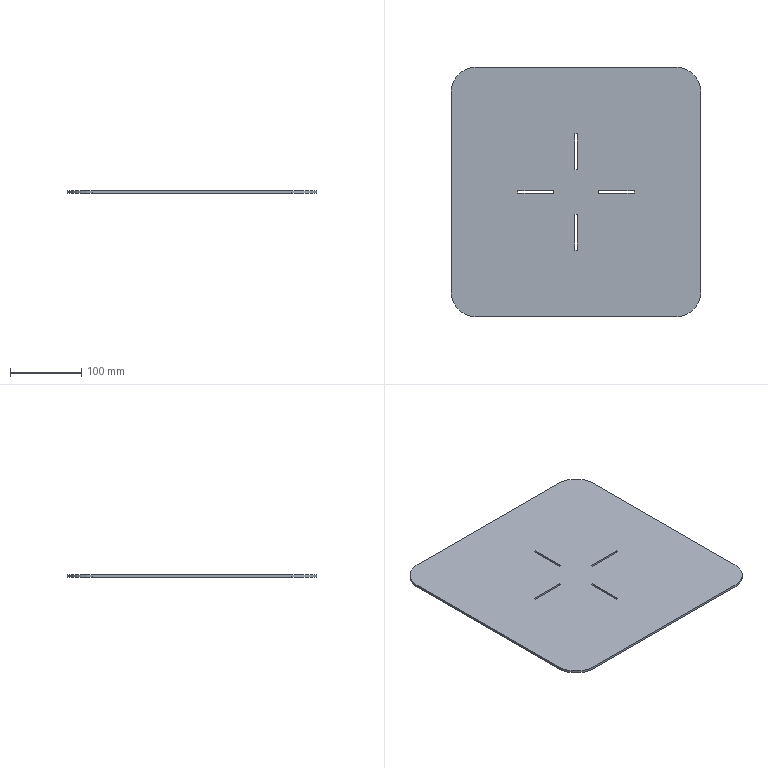Part | SolidWorks | features FlatPattern 1, SMBaseFlange 1, SheetMetal 1 | 1 solid | 26 faces | box 350 x 350 x 3.2 mm | volume 386587 mm3 | plane 22 | cylinder 4 | commonest cylinder face diameters 70 x4
STEP:
#1=CARTESIAN_POINT('',(163.93,-176.6,3.2));
#2=VERTEX_POINT('',#1);
#3=CARTESIAN_POINT('',(198.93,-141.6,3.2));
#4=VERTEX_POINT('',#3);
#5=CARTESIAN_POINT('',(163.93,-141.6,3.2));
#6=DIRECTION('',(0.,0.,1.));
#7=DIRECTION('',(1.,0.,0.));
#8=AXIS2_PLACEMENT_3D('',#5,#6,#7);
#9=CIRCLE('',#8,35.);
#10=EDGE_CURVE('',#2,#4,#9,.T.);
#11=ORIENTED_EDGE('',*,*,#10,.T.);
#12=CARTESIAN_POINT('',(198.93,138.4,3.2));
#13=VERTEX_POINT('',#12);
#14=CARTESIAN_POINT('',(198.93,-141.6,3.2));
#15=DIRECTION('',(0.,1.,0.));
#16=VECTOR('',#15,1000.);
#17=LINE('',#14,#16);
#18=EDGE_CURVE('',#4,#13,#17,.T.);
#19=ORIENTED_EDGE('',*,*,#18,.T.);
#20=CARTESIAN_POINT('',(163.93,173.4,3.2));
#21=VERTEX_POINT('',#20);
#22=CARTESIAN_POINT('',(163.93,138.4,3.2));
#23=DIRECTION('',(0.,0.,1.));
#24=DIRECTION('',(-1.,0.,0.));
#25=AXIS2_PLACEMENT_3D('',#22,#23,#24);
#26=CIRCLE('',#25,35.);
#27=EDGE_CURVE('',#13,#21,#26,.T.);
#28=ORIENTED_EDGE('',*,*,#27,.T.);
#29=CARTESIAN_POINT('',(-116.07,173.4,3.2));
#30=VERTEX_POINT('',#29);
#31=CARTESIAN_POINT('',(-116.07,173.4,3.2));
#32=DIRECTION('',(-1.,0.,0.));
#33=VECTOR('',#32,1000.);
#34=LINE('',#31,#33);
#35=EDGE_CURVE('',#21,#30,#34,.T.);
#36=ORIENTED_EDGE('',*,*,#35,.T.);
#37=CARTESIAN_POINT('',(-151.07,138.4,3.2));
#38=VERTEX_POINT('',#37);
#39=CARTESIAN_POINT('',(-116.07,138.4,3.2));
#40=DIRECTION('',(0.,0.,1.));
#41=DIRECTION('',(-1.,0.,0.));
#42=AXIS2_PLACEMENT_3D('',#39,#40,#41);
#43=CIRCLE('',#42,35.);
#44=EDGE_CURVE('',#30,#38,#43,.T.);
#45=ORIENTED_EDGE('',*,*,#44,.T.);
#46=CARTESIAN_POINT('',(-151.07,-141.6,3.2));
#47=VERTEX_POINT('',#46);
#48=CARTESIAN_POINT('',(-151.07,-141.6,3.2));
#49=DIRECTION('',(0.,-1.,0.));
#50=VECTOR('',#49,1000.);
#51=LINE('',#48,#50);
#52=EDGE_CURVE('',#38,#47,#51,.T.);
#53=ORIENTED_EDGE('',*,*,#52,.T.);
#54=CARTESIAN_POINT('',(-116.07,-176.6,3.2));
#55=VERTEX_POINT('',#54);
#56=CARTESIAN_POINT('',(-116.07,-141.6,3.2));
#57=DIRECTION('',(0.,0.,1.));
#58=DIRECTION('',(-1.,0.,0.));
#59=AXIS2_PLACEMENT_3D('',#56,#57,#58);
#60=CIRCLE('',#59,35.);
#61=EDGE_CURVE('',#47,#55,#60,.T.);
#62=ORIENTED_EDGE('',*,*,#61,.T.);
#63=CARTESIAN_POINT('',(-116.07,-176.6,3.2));
#64=DIRECTION('',(1.,0.,0.));
#65=VECTOR('',#64,1000.);
#66=LINE('',#63,#65);
#67=EDGE_CURVE('',#55,#2,#66,.T.);
#68=ORIENTED_EDGE('',*,*,#67,.T.);
#69=EDGE_LOOP('',(#11,#19,#28,#36,#45,#53,#62,#68));
#70=FACE_OUTER_BOUND('',#69,.T.);
#71=CARTESIAN_POINT('',(25.53,79.9,3.2));
#72=VERTEX_POINT('',#71);
#73=CARTESIAN_POINT('',(22.33,79.9,3.2));
#74=VERTEX_POINT('',#73);
#75=CARTESIAN_POINT('',(25.53,79.9,3.2));
#76=DIRECTION('',(-1.,0.,0.));
#77=VECTOR('',#76,1000.);
#78=LINE('',#75,#77);
#79=EDGE_CURVE('',#72,#74,#78,.T.);
#80=ORIENTED_EDGE('',*,*,#79,.F.);
#81=CARTESIAN_POINT('',(25.53,29.9,3.2));
#82=VERTEX_POINT('',#81);
#83=CARTESIAN_POINT('',(25.53,79.9,3.2));
#84=DIRECTION('',(0.,1.,0.));
#85=VECTOR('',#84,1000.);
#86=LINE('',#83,#85);
#87=EDGE_CURVE('',#82,#72,#86,.T.);
#88=ORIENTED_EDGE('',*,*,#87,.F.);
#89=CARTESIAN_POINT('',(22.33,29.9,3.2));
#90=VERTEX_POINT('',#89);
#91=CARTESIAN_POINT('',(25.53,29.9,3.2));
#92=DIRECTION('',(1.,0.,0.));
#93=VECTOR('',#92,1000.);
#94=LINE('',#91,#93);
#95=EDGE_CURVE('',#90,#82,#94,.T.);
#96=ORIENTED_EDGE('',*,*,#95,.F.);
#97=CARTESIAN_POINT('',(22.33,79.9,3.2));
#98=DIRECTION('',(0.,-1.,0.));
#99=VECTOR('',#98,1000.);
#100=LINE('',#97,#99);
#101=EDGE_CURVE('',#74,#90,#100,.T.);
#102=ORIENTED_EDGE('',*,*,#101,.F.);
#103=EDGE_LOOP('',(#80,#88,#96,#102));
#104=FACE_BOUND('',#103,.T.);
#105=CARTESIAN_POINT('',(105.43,0.,3.2));
#106=VERTEX_POINT('',#105);
#107=CARTESIAN_POINT('',(55.43,0.,3.2));
#108=VERTEX_POINT('',#107);
#109=CARTESIAN_POINT('',(105.43,0.,3.2));
#110=DIRECTION('',(-1.,0.,0.));
#111=VECTOR('',#110,1000.);
#112=LINE('',#109,#111);
#113=EDGE_CURVE('',#106,#108,#112,.T.);
#114=ORIENTED_EDGE('',*,*,#113,.F.);
#115=CARTESIAN_POINT('',(105.43,-3.2,3.2));
#116=VERTEX_POINT('',#115);
#117=CARTESIAN_POINT('',(105.43,0.,3.2));
#118=DIRECTION('',(0.,1.,0.));
#119=VECTOR('',#118,1000.);
#120=LINE('',#117,#119);
#121=EDGE_CURVE('',#116,#106,#120,.T.);
#122=ORIENTED_EDGE('',*,*,#121,.F.);
#123=CARTESIAN_POINT('',(55.43,-3.2,3.2));
#124=VERTEX_POINT('',#123);
#125=CARTESIAN_POINT('',(105.43,-3.2,3.2));
#126=DIRECTION('',(1.,0.,0.));
#127=VECTOR('',#126,1000.);
#128=LINE('',#125,#127);
#129=EDGE_CURVE('',#124,#116,#128,.T.);
#130=ORIENTED_EDGE('',*,*,#129,.F.);
#131=CARTESIAN_POINT('',(55.43,0.,3.2));
#132=DIRECTION('',(0.,-1.,0.));
#133=VECTOR('',#132,1000.);
#134=LINE('',#131,#133);
#135=EDGE_CURVE('',#108,#124,#134,.T.);
#136=ORIENTED_EDGE('',*,*,#135,.F.);
#137=EDGE_LOOP('',(#114,#122,#130,#136));
#138=FACE_BOUND('',#137,.T.);
#139=CARTESIAN_POINT('',(22.33,-83.1,3.2));
#140=VERTEX_POINT('',#139);
#141=CARTESIAN_POINT('',(25.53,-83.1,3.2));
#142=VERTEX_POINT('',#141);
#143=CARTESIAN_POINT('',(22.33,-83.1,3.2));
#144=DIRECTION('',(1.,0.,0.));
#145=VECTOR('',#144,1000.);
#146=LINE('',#143,#145);
#147=EDGE_CURVE('',#140,#142,#146,.T.);
#148=ORIENTED_EDGE('',*,*,#147,.F.);
#149=CARTESIAN_POINT('',(22.33,-33.1,3.2));
#150=VERTEX_POINT('',#149);
#151=CARTESIAN_POINT('',(22.33,-83.1,3.2));
#152=DIRECTION('',(0.,-1.,0.));
#153=VECTOR('',#152,1000.);
#154=LINE('',#151,#153);
#155=EDGE_CURVE('',#150,#140,#154,.T.);
#156=ORIENTED_EDGE('',*,*,#155,.F.);
#157=CARTESIAN_POINT('',(25.53,-33.1,3.2));
#158=VERTEX_POINT('',#157);
#159=CARTESIAN_POINT('',(22.33,-33.1,3.2));
#160=DIRECTION('',(-1.,0.,0.));
#161=VECTOR('',#160,1000.);
#162=LINE('',#159,#161);
#163=EDGE_CURVE('',#158,#150,#162,.T.);
#164=ORIENTED_EDGE('',*,*,#163,.F.);
#165=CARTESIAN_POINT('',(25.53,-83.1,3.2));
#166=DIRECTION('',(0.,1.,0.));
#167=VECTOR('',#166,1000.);
#168=LINE('',#165,#167);
#169=EDGE_CURVE('',#142,#158,#168,.T.);
#170=ORIENTED_EDGE('',*,*,#169,.F.);
#171=EDGE_LOOP('',(#148,#156,#164,#170));
#172=FACE_BOUND('',#171,.T.);
#173=CARTESIAN_POINT('',(-57.57,-3.2,3.2));
#174=VERTEX_POINT('',#173);
#175=CARTESIAN_POINT('',(-7.57,-3.2,3.2));
#176=VERTEX_POINT('',#175);
#177=CARTESIAN_POINT('',(-57.57,-3.2,3.2));
#178=DIRECTION('',(1.,0.,0.));
#179=VECTOR('',#178,1000.);
#180=LINE('',#177,#179);
#181=EDGE_CURVE('',#174,#176,#180,.T.);
#182=ORIENTED_EDGE('',*,*,#181,.F.);
#183=CARTESIAN_POINT('',(-57.57,0.,3.2));
#184=VERTEX_POINT('',#183);
#185=CARTESIAN_POINT('',(-57.57,-3.2,3.2));
#186=DIRECTION('',(0.,-1.,0.));
#187=VECTOR('',#186,1000.);
#188=LINE('',#185,#187);
#189=EDGE_CURVE('',#184,#174,#188,.T.);
#190=ORIENTED_EDGE('',*,*,#189,.F.);
#191=CARTESIAN_POINT('',(-7.57,0.,3.2));
#192=VERTEX_POINT('',#191);
#193=CARTESIAN_POINT('',(-57.57,0.,3.2));
#194=DIRECTION('',(-1.,0.,0.));
#195=VECTOR('',#194,1000.);
#196=LINE('',#193,#195);
#197=EDGE_CURVE('',#192,#184,#196,.T.);
#198=ORIENTED_EDGE('',*,*,#197,.F.);
#199=CARTESIAN_POINT('',(-7.57,-3.2,3.2));
#200=DIRECTION('',(0.,1.,0.));
#201=VECTOR('',#200,1000.);
#202=LINE('',#199,#201);
#203=EDGE_CURVE('',#176,#192,#202,.T.);
#204=ORIENTED_EDGE('',*,*,#203,.F.);
#205=EDGE_LOOP('',(#182,#190,#198,#204));
#206=FACE_BOUND('',#205,.T.);
#207=CARTESIAN_POINT('',(163.93,-141.6,3.2));
#208=DIRECTION('',(0.,0.,1.));
#209=DIRECTION('',(1.,0.,0.));
#210=AXIS2_PLACEMENT_3D('',#207,#208,#209);
#211=PLANE('',#210);
#212=ADVANCED_FACE('',(#70,#104,#138,#172,#206),#211,.T.);
#213=CARTESIAN_POINT('',(22.33,-33.1,0.));
#214=VERTEX_POINT('',#213);
#215=CARTESIAN_POINT('',(22.33,-83.1,0.));
#216=VERTEX_POINT('',#215);
#217=CARTESIAN_POINT('',(22.33,-83.1,0.));
#218=DIRECTION('',(0.,-1.,0.));
#219=VECTOR('',#218,1000.);
#220=LINE('',#217,#219);
#221=EDGE_CURVE('',#214,#216,#220,.T.);
#222=ORIENTED_EDGE('',*,*,#221,.T.);
#223=CARTESIAN_POINT('',(25.53,-83.1,0.));
#224=VERTEX_POINT('',#223);
#225=CARTESIAN_POINT('',(22.33,-83.1,0.));
#226=DIRECTION('',(1.,0.,0.));
#227=VECTOR('',#226,1000.);
#228=LINE('',#225,#227);
#229=EDGE_CURVE('',#216,#224,#228,.T.);
#230=ORIENTED_EDGE('',*,*,#229,.T.);
#231=CARTESIAN_POINT('',(25.53,-33.1,0.));
#232=VERTEX_POINT('',#231);
#233=CARTESIAN_POINT('',(25.53,-83.1,0.));
#234=DIRECTION('',(0.,1.,0.));
#235=VECTOR('',#234,1000.);
#236=LINE('',#233,#235);
#237=EDGE_CURVE('',#224,#232,#236,.T.);
#238=ORIENTED_EDGE('',*,*,#237,.T.);
#239=CARTESIAN_POINT('',(22.33,-33.1,0.));
#240=DIRECTION('',(-1.,0.,0.));
#241=VECTOR('',#240,1000.);
#242=LINE('',#239,#241);
#243=EDGE_CURVE('',#232,#214,#242,.T.);
#244=ORIENTED_EDGE('',*,*,#243,.T.);
#245=EDGE_LOOP('',(#222,#230,#238,#244));
#246=FACE_BOUND('',#245,.T.);
#247=CARTESIAN_POINT('',(25.53,29.9,0.));
#248=VERTEX_POINT('',#247);
#249=CARTESIAN_POINT('',(25.53,79.9,0.));
#250=VERTEX_POINT('',#249);
#251=CARTESIAN_POINT('',(25.53,79.9,0.));
#252=DIRECTION('',(0.,1.,0.));
#253=VECTOR('',#252,1000.);
#254=LINE('',#251,#253);
#255=EDGE_CURVE('',#248,#250,#254,.T.);
#256=ORIENTED_EDGE('',*,*,#255,.T.);
#257=CARTESIAN_POINT('',(22.33,79.9,0.));
#258=VERTEX_POINT('',#257);
#259=CARTESIAN_POINT('',(25.53,79.9,0.));
#260=DIRECTION('',(-1.,0.,0.));
#261=VECTOR('',#260,1000.);
#262=LINE('',#259,#261);
#263=EDGE_CURVE('',#250,#258,#262,.T.);
#264=ORIENTED_EDGE('',*,*,#263,.T.);
#265=CARTESIAN_POINT('',(22.33,29.9,0.));
#266=VERTEX_POINT('',#265);
#267=CARTESIAN_POINT('',(22.33,79.9,0.));
#268=DIRECTION('',(0.,-1.,0.));
#269=VECTOR('',#268,1000.);
#270=LINE('',#267,#269);
#271=EDGE_CURVE('',#258,#266,#270,.T.);
#272=ORIENTED_EDGE('',*,*,#271,.T.);
#273=CARTESIAN_POINT('',(25.53,29.9,0.));
#274=DIRECTION('',(1.,0.,0.));
#275=VECTOR('',#274,1000.);
#276=LINE('',#273,#275);
#277=EDGE_CURVE('',#266,#248,#276,.T.);
#278=ORIENTED_EDGE('',*,*,#277,.T.);
#279=EDGE_LOOP('',(#256,#264,#272,#278));
#280=FACE_BOUND('',#279,.T.);
#281=CARTESIAN_POINT('',(163.93,-176.6,0.));
#282=VERTEX_POINT('',#281);
#283=CARTESIAN_POINT('',(198.93,-141.6,0.));
#284=VERTEX_POINT('',#283);
#285=CARTESIAN_POINT('',(163.93,-141.6,0.));
#286=DIRECTION('',(0.,0.,1.));
#287=DIRECTION('',(1.,0.,0.));
#288=AXIS2_PLACEMENT_3D('',#285,#286,#287);
#289=CIRCLE('',#288,35.);
#290=EDGE_CURVE('',#282,#284,#289,.T.);
#291=ORIENTED_EDGE('',*,*,#290,.F.);
#292=CARTESIAN_POINT('',(-116.07,-176.6,0.));
#293=VERTEX_POINT('',#292);
#294=CARTESIAN_POINT('',(-116.07,-176.6,0.));
#295=DIRECTION('',(1.,0.,0.));
#296=VECTOR('',#295,1000.);
#297=LINE('',#294,#296);
#298=EDGE_CURVE('',#293,#282,#297,.T.);
#299=ORIENTED_EDGE('',*,*,#298,.F.);
#300=CARTESIAN_POINT('',(-151.07,-141.6,0.));
#301=VERTEX_POINT('',#300);
#302=CARTESIAN_POINT('',(-116.07,-141.6,0.));
#303=DIRECTION('',(0.,0.,1.));
#304=DIRECTION('',(-1.,0.,0.));
#305=AXIS2_PLACEMENT_3D('',#302,#303,#304);
#306=CIRCLE('',#305,35.);
#307=EDGE_CURVE('',#301,#293,#306,.T.);
#308=ORIENTED_EDGE('',*,*,#307,.F.);
#309=CARTESIAN_POINT('',(-151.07,138.4,0.));
#310=VERTEX_POINT('',#309);
#311=CARTESIAN_POINT('',(-151.07,-141.6,0.));
#312=DIRECTION('',(0.,-1.,0.));
#313=VECTOR('',#312,1000.);
#314=LINE('',#311,#313);
#315=EDGE_CURVE('',#310,#301,#314,.T.);
#316=ORIENTED_EDGE('',*,*,#315,.F.);
#317=CARTESIAN_POINT('',(-116.07,173.4,0.));
#318=VERTEX_POINT('',#317);
#319=CARTESIAN_POINT('',(-116.07,138.4,0.));
#320=DIRECTION('',(0.,0.,1.));
#321=DIRECTION('',(-1.,0.,0.));
#322=AXIS2_PLACEMENT_3D('',#319,#320,#321);
#323=CIRCLE('',#322,35.);
#324=EDGE_CURVE('',#318,#310,#323,.T.);
#325=ORIENTED_EDGE('',*,*,#324,.F.);
#326=CARTESIAN_POINT('',(163.93,173.4,0.));
#327=VERTEX_POINT('',#326);
#328=CARTESIAN_POINT('',(-116.07,173.4,0.));
#329=DIRECTION('',(-1.,0.,0.));
#330=VECTOR('',#329,1000.);
#331=LINE('',#328,#330);
#332=EDGE_CURVE('',#327,#318,#331,.T.);
#333=ORIENTED_EDGE('',*,*,#332,.F.);
#334=CARTESIAN_POINT('',(198.93,138.4,0.));
#335=VERTEX_POINT('',#334);
#336=CARTESIAN_POINT('',(163.93,138.4,0.));
#337=DIRECTION('',(0.,0.,1.));
#338=DIRECTION('',(-1.,0.,0.));
#339=AXIS2_PLACEMENT_3D('',#336,#337,#338);
#340=CIRCLE('',#339,35.);
#341=EDGE_CURVE('',#335,#327,#340,.T.);
#342=ORIENTED_EDGE('',*,*,#341,.F.);
#343=CARTESIAN_POINT('',(198.93,-141.6,0.));
#344=DIRECTION('',(0.,1.,0.));
#345=VECTOR('',#344,1000.);
#346=LINE('',#343,#345);
#347=EDGE_CURVE('',#284,#335,#346,.T.);
#348=ORIENTED_EDGE('',*,*,#347,.F.);
#349=EDGE_LOOP('',(#291,#299,#308,#316,#325,#333,#342,#348));
#350=FACE_OUTER_BOUND('',#349,.T.);
#351=CARTESIAN_POINT('',(105.43,-3.2,0.));
#352=VERTEX_POINT('',#351);
#353=CARTESIAN_POINT('',(105.43,0.,0.));
#354=VERTEX_POINT('',#353);
#355=CARTESIAN_POINT('',(105.43,0.,0.));
#356=DIRECTION('',(0.,1.,0.));
#357=VECTOR('',#356,1000.);
#358=LINE('',#355,#357);
#359=EDGE_CURVE('',#352,#354,#358,.T.);
#360=ORIENTED_EDGE('',*,*,#359,.T.);
#361=CARTESIAN_POINT('',(55.43,0.,0.));
#362=VERTEX_POINT('',#361);
#363=CARTESIAN_POINT('',(105.43,0.,0.));
#364=DIRECTION('',(-1.,0.,0.));
#365=VECTOR('',#364,1000.);
#366=LINE('',#363,#365);
#367=EDGE_CURVE('',#354,#362,#366,.T.);
#368=ORIENTED_EDGE('',*,*,#367,.T.);
#369=CARTESIAN_POINT('',(55.43,-3.2,0.));
#370=VERTEX_POINT('',#369);
#371=CARTESIAN_POINT('',(55.43,0.,0.));
#372=DIRECTION('',(0.,-1.,0.));
#373=VECTOR('',#372,1000.);
#374=LINE('',#371,#373);
#375=EDGE_CURVE('',#362,#370,#374,.T.);
#376=ORIENTED_EDGE('',*,*,#375,.T.);
#377=CARTESIAN_POINT('',(105.43,-3.2,0.));
#378=DIRECTION('',(1.,0.,0.));
#379=VECTOR('',#378,1000.);
#380=LINE('',#377,#379);
#381=EDGE_CURVE('',#370,#352,#380,.T.);
#382=ORIENTED_EDGE('',*,*,#381,.T.);
#383=EDGE_LOOP('',(#360,#368,#376,#382));
#384=FACE_BOUND('',#383,.T.);
#385=CARTESIAN_POINT('',(-57.57,0.,0.));
#386=VERTEX_POINT('',#385);
#387=CARTESIAN_POINT('',(-57.57,-3.2,0.));
#388=VERTEX_POINT('',#387);
#389=CARTESIAN_POINT('',(-57.57,-3.2,0.));
#390=DIRECTION('',(0.,-1.,0.));
#391=VECTOR('',#390,1000.);
#392=LINE('',#389,#391);
#393=EDGE_CURVE('',#386,#388,#392,.T.);
#394=ORIENTED_EDGE('',*,*,#393,.T.);
#395=CARTESIAN_POINT('',(-7.57,-3.2,0.));
#396=VERTEX_POINT('',#395);
#397=CARTESIAN_POINT('',(-57.57,-3.2,0.));
#398=DIRECTION('',(1.,0.,0.));
#399=VECTOR('',#398,1000.);
#400=LINE('',#397,#399);
#401=EDGE_CURVE('',#388,#396,#400,.T.);
#402=ORIENTED_EDGE('',*,*,#401,.T.);
#403=CARTESIAN_POINT('',(-7.57,0.,0.));
#404=VERTEX_POINT('',#403);
#405=CARTESIAN_POINT('',(-7.57,-3.2,0.));
#406=DIRECTION('',(0.,1.,0.));
#407=VECTOR('',#406,1000.);
#408=LINE('',#405,#407);
#409=EDGE_CURVE('',#396,#404,#408,.T.);
#410=ORIENTED_EDGE('',*,*,#409,.T.);
#411=CARTESIAN_POINT('',(-57.57,0.,0.));
#412=DIRECTION('',(-1.,0.,0.));
#413=VECTOR('',#412,1000.);
#414=LINE('',#411,#413);
#415=EDGE_CURVE('',#404,#386,#414,.T.);
#416=ORIENTED_EDGE('',*,*,#415,.T.);
#417=EDGE_LOOP('',(#394,#402,#410,#416));
#418=FACE_BOUND('',#417,.T.);
#419=CARTESIAN_POINT('',(163.93,-141.6,0.));
#420=DIRECTION('',(0.,0.,1.));
#421=DIRECTION('',(1.,0.,0.));
#422=AXIS2_PLACEMENT_3D('',#419,#420,#421);
#423=PLANE('',#422);
#424=ADVANCED_FACE('',(#246,#280,#350,#384,#418),#423,.F.);
#425=ORIENTED_EDGE('',*,*,#290,.T.);
#426=CARTESIAN_POINT('',(198.93,-141.6,3.2));
#427=DIRECTION('',(0.,0.,-1.));
#428=VECTOR('',#427,1000.);
#429=LINE('',#426,#428);
#430=EDGE_CURVE('',#4,#284,#429,.T.);
#431=ORIENTED_EDGE('',*,*,#430,.F.);
#432=ORIENTED_EDGE('',*,*,#10,.F.);
#433=CARTESIAN_POINT('',(163.93,-176.6,3.2));
#434=DIRECTION('',(0.,0.,-1.));
#435=VECTOR('',#434,1000.);
#436=LINE('',#433,#435);
#437=EDGE_CURVE('',#2,#282,#436,.T.);
#438=ORIENTED_EDGE('',*,*,#437,.T.);
#439=EDGE_LOOP('',(#425,#431,#432,#438));
#440=FACE_OUTER_BOUND('',#439,.T.);
#441=CARTESIAN_POINT('',(163.93,-141.6,3.2));
#442=DIRECTION('',(0.,0.,-1.));
#443=DIRECTION('',(-1.,0.,0.));
#444=AXIS2_PLACEMENT_3D('',#441,#442,#443);
#445=CYLINDRICAL_SURFACE('',#444,35.);
#446=ADVANCED_FACE('',(#440),#445,.T.);
#447=ORIENTED_EDGE('',*,*,#347,.T.);
#448=CARTESIAN_POINT('',(198.93,138.4,3.2));
#449=DIRECTION('',(0.,0.,-1.));
#450=VECTOR('',#449,1000.);
#451=LINE('',#448,#450);
#452=EDGE_CURVE('',#13,#335,#451,.T.);
#453=ORIENTED_EDGE('',*,*,#452,.F.);
#454=ORIENTED_EDGE('',*,*,#18,.F.);
#455=ORIENTED_EDGE('',*,*,#430,.T.);
#456=EDGE_LOOP('',(#447,#453,#454,#455));
#457=FACE_OUTER_BOUND('',#456,.T.);
#458=CARTESIAN_POINT('',(198.93,-141.6,3.2));
#459=DIRECTION('',(-1.,0.,0.));
#460=DIRECTION('',(0.,-1.,0.));
#461=AXIS2_PLACEMENT_3D('',#458,#459,#460);
#462=PLANE('',#461);
#463=ADVANCED_FACE('',(#457),#462,.F.);
#464=ORIENTED_EDGE('',*,*,#341,.T.);
#465=CARTESIAN_POINT('',(163.93,173.4,3.2));
#466=DIRECTION('',(0.,0.,-1.));
#467=VECTOR('',#466,1000.);
#468=LINE('',#465,#467);
#469=EDGE_CURVE('',#21,#327,#468,.T.);
#470=ORIENTED_EDGE('',*,*,#469,.F.);
#471=ORIENTED_EDGE('',*,*,#27,.F.);
#472=ORIENTED_EDGE('',*,*,#452,.T.);
#473=EDGE_LOOP('',(#464,#470,#471,#472));
#474=FACE_OUTER_BOUND('',#473,.T.);
#475=CARTESIAN_POINT('',(163.93,138.4,3.2));
#476=DIRECTION('',(0.,0.,-1.));
#477=DIRECTION('',(-1.,0.,0.));
#478=AXIS2_PLACEMENT_3D('',#475,#476,#477);
#479=CYLINDRICAL_SURFACE('',#478,35.);
#480=ADVANCED_FACE('',(#474),#479,.T.);
#481=ORIENTED_EDGE('',*,*,#332,.T.);
#482=CARTESIAN_POINT('',(-116.07,173.4,3.2));
#483=DIRECTION('',(0.,0.,-1.));
#484=VECTOR('',#483,1000.);
#485=LINE('',#482,#484);
#486=EDGE_CURVE('',#30,#318,#485,.T.);
#487=ORIENTED_EDGE('',*,*,#486,.F.);
#488=ORIENTED_EDGE('',*,*,#35,.F.);
#489=ORIENTED_EDGE('',*,*,#469,.T.);
#490=EDGE_LOOP('',(#481,#487,#488,#489));
#491=FACE_OUTER_BOUND('',#490,.T.);
#492=CARTESIAN_POINT('',(-116.07,173.4,3.2));
#493=DIRECTION('',(0.,-1.,0.));
#494=DIRECTION('',(0.,0.,-1.));
#495=AXIS2_PLACEMENT_3D('',#492,#493,#494);
#496=PLANE('',#495);
#497=ADVANCED_FACE('',(#491),#496,.F.);
#498=ORIENTED_EDGE('',*,*,#324,.T.);
#499=CARTESIAN_POINT('',(-151.07,138.4,3.2));
#500=DIRECTION('',(0.,0.,-1.));
#501=VECTOR('',#500,1000.);
#502=LINE('',#499,#501);
#503=EDGE_CURVE('',#38,#310,#502,.T.);
#504=ORIENTED_EDGE('',*,*,#503,.F.);
#505=ORIENTED_EDGE('',*,*,#44,.F.);
#506=ORIENTED_EDGE('',*,*,#486,.T.);
#507=EDGE_LOOP('',(#498,#504,#505,#506));
#508=FACE_OUTER_BOUND('',#507,.T.);
#509=CARTESIAN_POINT('',(-116.07,138.4,3.2));
#510=DIRECTION('',(0.,0.,-1.));
#511=DIRECTION('',(-1.,0.,0.));
#512=AXIS2_PLACEMENT_3D('',#509,#510,#511);
#513=CYLINDRICAL_SURFACE('',#512,35.);
#514=ADVANCED_FACE('',(#508),#513,.T.);
#515=ORIENTED_EDGE('',*,*,#315,.T.);
#516=CARTESIAN_POINT('',(-151.07,-141.6,3.2));
#517=DIRECTION('',(0.,0.,-1.));
#518=VECTOR('',#517,1000.);
#519=LINE('',#516,#518);
#520=EDGE_CURVE('',#47,#301,#519,.T.);
#521=ORIENTED_EDGE('',*,*,#520,.F.);
#522=ORIENTED_EDGE('',*,*,#52,.F.);
#523=ORIENTED_EDGE('',*,*,#503,.T.);
#524=EDGE_LOOP('',(#515,#521,#522,#523));
#525=FACE_OUTER_BOUND('',#524,.T.);
#526=CARTESIAN_POINT('',(-151.07,-141.6,3.2));
#527=DIRECTION('',(1.,0.,0.));
#528=DIRECTION('',(0.,0.,-1.));
#529=AXIS2_PLACEMENT_3D('',#526,#527,#528);
#530=PLANE('',#529);
#531=ADVANCED_FACE('',(#525),#530,.F.);
#532=ORIENTED_EDGE('',*,*,#307,.T.);
#533=CARTESIAN_POINT('',(-116.07,-176.6,3.2));
#534=DIRECTION('',(0.,0.,-1.));
#535=VECTOR('',#534,1000.);
#536=LINE('',#533,#535);
#537=EDGE_CURVE('',#55,#293,#536,.T.);
#538=ORIENTED_EDGE('',*,*,#537,.F.);
#539=ORIENTED_EDGE('',*,*,#61,.F.);
#540=ORIENTED_EDGE('',*,*,#520,.T.);
#541=EDGE_LOOP('',(#532,#538,#539,#540));
#542=FACE_OUTER_BOUND('',#541,.T.);
#543=CARTESIAN_POINT('',(-116.07,-141.6,3.2));
#544=DIRECTION('',(0.,0.,-1.));
#545=DIRECTION('',(-1.,0.,0.));
#546=AXIS2_PLACEMENT_3D('',#543,#544,#545);
#547=CYLINDRICAL_SURFACE('',#546,35.);
#548=ADVANCED_FACE('',(#542),#547,.T.);
#549=ORIENTED_EDGE('',*,*,#298,.T.);
#550=ORIENTED_EDGE('',*,*,#437,.F.);
#551=ORIENTED_EDGE('',*,*,#67,.F.);
#552=ORIENTED_EDGE('',*,*,#537,.T.);
#553=EDGE_LOOP('',(#549,#550,#551,#552));
#554=FACE_OUTER_BOUND('',#553,.T.);
#555=CARTESIAN_POINT('',(-116.07,-176.6,3.2));
#556=DIRECTION('',(0.,1.,0.));
#557=DIRECTION('',(0.,0.,1.));
#558=AXIS2_PLACEMENT_3D('',#555,#556,#557);
#559=PLANE('',#558);
#560=ADVANCED_FACE('',(#554),#559,.F.);
#561=ORIENTED_EDGE('',*,*,#255,.F.);
#562=CARTESIAN_POINT('',(25.53,29.9,3.2));
#563=DIRECTION('',(0.,0.,-1.));
#564=VECTOR('',#563,1000.);
#565=LINE('',#562,#564);
#566=EDGE_CURVE('',#82,#248,#565,.T.);
#567=ORIENTED_EDGE('',*,*,#566,.F.);
#568=ORIENTED_EDGE('',*,*,#87,.T.);
#569=CARTESIAN_POINT('',(25.53,79.9,3.2));
#570=DIRECTION('',(0.,0.,-1.));
#571=VECTOR('',#570,1000.);
#572=LINE('',#569,#571);
#573=EDGE_CURVE('',#72,#250,#572,.T.);
#574=ORIENTED_EDGE('',*,*,#573,.T.);
#575=EDGE_LOOP('',(#561,#567,#568,#574));
#576=FACE_OUTER_BOUND('',#575,.T.);
#577=CARTESIAN_POINT('',(25.53,79.9,3.2));
#578=DIRECTION('',(-1.,0.,0.));
#579=DIRECTION('',(0.,0.,1.));
#580=AXIS2_PLACEMENT_3D('',#577,#578,#579);
#581=PLANE('',#580);
#582=ADVANCED_FACE('',(#576),#581,.T.);
#583=ORIENTED_EDGE('',*,*,#263,.F.);
#584=ORIENTED_EDGE('',*,*,#573,.F.);
#585=ORIENTED_EDGE('',*,*,#79,.T.);
#586=CARTESIAN_POINT('',(22.33,79.9,3.2));
#587=DIRECTION('',(0.,0.,-1.));
#588=VECTOR('',#587,1000.);
#589=LINE('',#586,#588);
#590=EDGE_CURVE('',#74,#258,#589,.T.);
#591=ORIENTED_EDGE('',*,*,#590,.T.);
#592=EDGE_LOOP('',(#583,#584,#585,#591));
#593=FACE_OUTER_BOUND('',#592,.T.);
#594=CARTESIAN_POINT('',(25.53,79.9,3.2));
#595=DIRECTION('',(0.,-1.,0.));
#596=DIRECTION('',(0.,0.,-1.));
#597=AXIS2_PLACEMENT_3D('',#594,#595,#596);
#598=PLANE('',#597);
#599=ADVANCED_FACE('',(#593),#598,.T.);
#600=ORIENTED_EDGE('',*,*,#271,.F.);
#601=ORIENTED_EDGE('',*,*,#590,.F.);
#602=ORIENTED_EDGE('',*,*,#101,.T.);
#603=CARTESIAN_POINT('',(22.33,29.9,3.2));
#604=DIRECTION('',(0.,0.,-1.));
#605=VECTOR('',#604,1000.);
#606=LINE('',#603,#605);
#607=EDGE_CURVE('',#90,#266,#606,.T.);
#608=ORIENTED_EDGE('',*,*,#607,.T.);
#609=EDGE_LOOP('',(#600,#601,#602,#608));
#610=FACE_OUTER_BOUND('',#609,.T.);
#611=CARTESIAN_POINT('',(22.33,79.9,3.2));
#612=DIRECTION('',(1.,0.,0.));
#613=DIRECTION('',(0.,0.,-1.));
#614=AXIS2_PLACEMENT_3D('',#611,#612,#613);
#615=PLANE('',#614);
#616=ADVANCED_FACE('',(#610),#615,.T.);
#617=ORIENTED_EDGE('',*,*,#277,.F.);
#618=ORIENTED_EDGE('',*,*,#607,.F.);
#619=ORIENTED_EDGE('',*,*,#95,.T.);
#620=ORIENTED_EDGE('',*,*,#566,.T.);
#621=EDGE_LOOP('',(#617,#618,#619,#620));
#622=FACE_OUTER_BOUND('',#621,.T.);
#623=CARTESIAN_POINT('',(25.53,29.9,3.2));
#624=DIRECTION('',(0.,1.,0.));
#625=DIRECTION('',(0.,0.,1.));
#626=AXIS2_PLACEMENT_3D('',#623,#624,#625);
#627=PLANE('',#626);
#628=ADVANCED_FACE('',(#622),#627,.T.);
#629=ORIENTED_EDGE('',*,*,#359,.F.);
#630=CARTESIAN_POINT('',(105.43,-3.2,3.2));
#631=DIRECTION('',(0.,0.,-1.));
#632=VECTOR('',#631,1000.);
#633=LINE('',#630,#632);
#634=EDGE_CURVE('',#116,#352,#633,.T.);
#635=ORIENTED_EDGE('',*,*,#634,.F.);
#636=ORIENTED_EDGE('',*,*,#121,.T.);
#637=CARTESIAN_POINT('',(105.43,0.,3.2));
#638=DIRECTION('',(0.,0.,-1.));
#639=VECTOR('',#638,1000.);
#640=LINE('',#637,#639);
#641=EDGE_CURVE('',#106,#354,#640,.T.);
#642=ORIENTED_EDGE('',*,*,#641,.T.);
#643=EDGE_LOOP('',(#629,#635,#636,#642));
#644=FACE_OUTER_BOUND('',#643,.T.);
#645=CARTESIAN_POINT('',(105.43,0.,3.2));
#646=DIRECTION('',(-1.,0.,0.));
#647=DIRECTION('',(0.,0.,1.));
#648=AXIS2_PLACEMENT_3D('',#645,#646,#647);
#649=PLANE('',#648);
#650=ADVANCED_FACE('',(#644),#649,.T.);
#651=ORIENTED_EDGE('',*,*,#367,.F.);
#652=ORIENTED_EDGE('',*,*,#641,.F.);
#653=ORIENTED_EDGE('',*,*,#113,.T.);
#654=CARTESIAN_POINT('',(55.43,0.,3.2));
#655=DIRECTION('',(0.,0.,-1.));
#656=VECTOR('',#655,1000.);
#657=LINE('',#654,#656);
#658=EDGE_CURVE('',#108,#362,#657,.T.);
#659=ORIENTED_EDGE('',*,*,#658,.T.);
#660=EDGE_LOOP('',(#651,#652,#653,#659));
#661=FACE_OUTER_BOUND('',#660,.T.);
#662=CARTESIAN_POINT('',(105.43,0.,3.2));
#663=DIRECTION('',(0.,-1.,0.));
#664=DIRECTION('',(0.,0.,-1.));
#665=AXIS2_PLACEMENT_3D('',#662,#663,#664);
#666=PLANE('',#665);
#667=ADVANCED_FACE('',(#661),#666,.T.);
#668=ORIENTED_EDGE('',*,*,#375,.F.);
#669=ORIENTED_EDGE('',*,*,#658,.F.);
#670=ORIENTED_EDGE('',*,*,#135,.T.);
#671=CARTESIAN_POINT('',(55.43,-3.2,3.2));
#672=DIRECTION('',(0.,0.,-1.));
#673=VECTOR('',#672,1000.);
#674=LINE('',#671,#673);
#675=EDGE_CURVE('',#124,#370,#674,.T.);
#676=ORIENTED_EDGE('',*,*,#675,.T.);
#677=EDGE_LOOP('',(#668,#669,#670,#676));
#678=FACE_OUTER_BOUND('',#677,.T.);
#679=CARTESIAN_POINT('',(55.43,0.,3.2));
#680=DIRECTION('',(1.,0.,0.));
#681=DIRECTION('',(0.,0.,-1.));
#682=AXIS2_PLACEMENT_3D('',#679,#680,#681);
#683=PLANE('',#682);
#684=ADVANCED_FACE('',(#678),#683,.T.);
#685=ORIENTED_EDGE('',*,*,#381,.F.);
#686=ORIENTED_EDGE('',*,*,#675,.F.);
#687=ORIENTED_EDGE('',*,*,#129,.T.);
#688=ORIENTED_EDGE('',*,*,#634,.T.);
#689=EDGE_LOOP('',(#685,#686,#687,#688));
#690=FACE_OUTER_BOUND('',#689,.T.);
#691=CARTESIAN_POINT('',(105.43,-3.2,3.2));
#692=DIRECTION('',(0.,1.,0.));
#693=DIRECTION('',(0.,0.,1.));
#694=AXIS2_PLACEMENT_3D('',#691,#692,#693);
#695=PLANE('',#694);
#696=ADVANCED_FACE('',(#690),#695,.T.);
#697=ORIENTED_EDGE('',*,*,#221,.F.);
#698=CARTESIAN_POINT('',(22.33,-33.1,3.2));
#699=DIRECTION('',(0.,0.,-1.));
#700=VECTOR('',#699,1000.);
#701=LINE('',#698,#700);
#702=EDGE_CURVE('',#150,#214,#701,.T.);
#703=ORIENTED_EDGE('',*,*,#702,.F.);
#704=ORIENTED_EDGE('',*,*,#155,.T.);
#705=CARTESIAN_POINT('',(22.33,-83.1,3.2));
#706=DIRECTION('',(0.,0.,-1.));
#707=VECTOR('',#706,1000.);
#708=LINE('',#705,#707);
#709=EDGE_CURVE('',#140,#216,#708,.T.);
#710=ORIENTED_EDGE('',*,*,#709,.T.);
#711=EDGE_LOOP('',(#697,#703,#704,#710));
#712=FACE_OUTER_BOUND('',#711,.T.);
#713=CARTESIAN_POINT('',(22.33,-83.1,3.2));
#714=DIRECTION('',(1.,0.,0.));
#715=DIRECTION('',(0.,0.,-1.));
#716=AXIS2_PLACEMENT_3D('',#713,#714,#715);
#717=PLANE('',#716);
#718=ADVANCED_FACE('',(#712),#717,.T.);
#719=ORIENTED_EDGE('',*,*,#229,.F.);
#720=ORIENTED_EDGE('',*,*,#709,.F.);
#721=ORIENTED_EDGE('',*,*,#147,.T.);
#722=CARTESIAN_POINT('',(25.53,-83.1,3.2));
#723=DIRECTION('',(0.,0.,-1.));
#724=VECTOR('',#723,1000.);
#725=LINE('',#722,#724);
#726=EDGE_CURVE('',#142,#224,#725,.T.);
#727=ORIENTED_EDGE('',*,*,#726,.T.);
#728=EDGE_LOOP('',(#719,#720,#721,#727));
#729=FACE_OUTER_BOUND('',#728,.T.);
#730=CARTESIAN_POINT('',(22.33,-83.1,3.2));
#731=DIRECTION('',(0.,1.,0.));
#732=DIRECTION('',(0.,0.,1.));
#733=AXIS2_PLACEMENT_3D('',#730,#731,#732);
#734=PLANE('',#733);
#735=ADVANCED_FACE('',(#729),#734,.T.);
#736=ORIENTED_EDGE('',*,*,#237,.F.);
#737=ORIENTED_EDGE('',*,*,#726,.F.);
#738=ORIENTED_EDGE('',*,*,#169,.T.);
#739=CARTESIAN_POINT('',(25.53,-33.1,3.2));
#740=DIRECTION('',(0.,0.,-1.));
#741=VECTOR('',#740,1000.);
#742=LINE('',#739,#741);
#743=EDGE_CURVE('',#158,#232,#742,.T.);
#744=ORIENTED_EDGE('',*,*,#743,.T.);
#745=EDGE_LOOP('',(#736,#737,#738,#744));
#746=FACE_OUTER_BOUND('',#745,.T.);
#747=CARTESIAN_POINT('',(25.53,-83.1,3.2));
#748=DIRECTION('',(-1.,0.,0.));
#749=DIRECTION('',(0.,0.,1.));
#750=AXIS2_PLACEMENT_3D('',#747,#748,#749);
#751=PLANE('',#750);
#752=ADVANCED_FACE('',(#746),#751,.T.);
#753=ORIENTED_EDGE('',*,*,#243,.F.);
#754=ORIENTED_EDGE('',*,*,#743,.F.);
#755=ORIENTED_EDGE('',*,*,#163,.T.);
#756=ORIENTED_EDGE('',*,*,#702,.T.);
#757=EDGE_LOOP('',(#753,#754,#755,#756));
#758=FACE_OUTER_BOUND('',#757,.T.);
#759=CARTESIAN_POINT('',(22.33,-33.1,3.2));
#760=DIRECTION('',(0.,-1.,0.));
#761=DIRECTION('',(0.,0.,-1.));
#762=AXIS2_PLACEMENT_3D('',#759,#760,#761);
#763=PLANE('',#762);
#764=ADVANCED_FACE('',(#758),#763,.T.);
#765=ORIENTED_EDGE('',*,*,#393,.F.);
#766=CARTESIAN_POINT('',(-57.57,0.,3.2));
#767=DIRECTION('',(0.,0.,-1.));
#768=VECTOR('',#767,1000.);
#769=LINE('',#766,#768);
#770=EDGE_CURVE('',#184,#386,#769,.T.);
#771=ORIENTED_EDGE('',*,*,#770,.F.);
#772=ORIENTED_EDGE('',*,*,#189,.T.);
#773=CARTESIAN_POINT('',(-57.57,-3.2,3.2));
#774=DIRECTION('',(0.,0.,-1.));
#775=VECTOR('',#774,1000.);
#776=LINE('',#773,#775);
#777=EDGE_CURVE('',#174,#388,#776,.T.);
#778=ORIENTED_EDGE('',*,*,#777,.T.);
#779=EDGE_LOOP('',(#765,#771,#772,#778));
#780=FACE_OUTER_BOUND('',#779,.T.);
#781=CARTESIAN_POINT('',(-57.57,-3.2,3.2));
#782=DIRECTION('',(1.,0.,0.));
#783=DIRECTION('',(0.,0.,-1.));
#784=AXIS2_PLACEMENT_3D('',#781,#782,#783);
#785=PLANE('',#784);
#786=ADVANCED_FACE('',(#780),#785,.T.);
#787=ORIENTED_EDGE('',*,*,#401,.F.);
#788=ORIENTED_EDGE('',*,*,#777,.F.);
#789=ORIENTED_EDGE('',*,*,#181,.T.);
#790=CARTESIAN_POINT('',(-7.57,-3.2,3.2));
#791=DIRECTION('',(0.,0.,-1.));
#792=VECTOR('',#791,1000.);
#793=LINE('',#790,#792);
#794=EDGE_CURVE('',#176,#396,#793,.T.);
#795=ORIENTED_EDGE('',*,*,#794,.T.);
#796=EDGE_LOOP('',(#787,#788,#789,#795));
#797=FACE_OUTER_BOUND('',#796,.T.);
#798=CARTESIAN_POINT('',(-57.57,-3.2,3.2));
#799=DIRECTION('',(0.,1.,0.));
#800=DIRECTION('',(0.,0.,1.));
#801=AXIS2_PLACEMENT_3D('',#798,#799,#800);
#802=PLANE('',#801);
#803=ADVANCED_FACE('',(#797),#802,.T.);
#804=ORIENTED_EDGE('',*,*,#409,.F.);
#805=ORIENTED_EDGE('',*,*,#794,.F.);
#806=ORIENTED_EDGE('',*,*,#203,.T.);
#807=CARTESIAN_POINT('',(-7.57,0.,3.2));
#808=DIRECTION('',(0.,0.,-1.));
#809=VECTOR('',#808,1000.);
#810=LINE('',#807,#809);
#811=EDGE_CURVE('',#192,#404,#810,.T.);
#812=ORIENTED_EDGE('',*,*,#811,.T.);
#813=EDGE_LOOP('',(#804,#805,#806,#812));
#814=FACE_OUTER_BOUND('',#813,.T.);
#815=CARTESIAN_POINT('',(-7.57,-3.2,3.2));
#816=DIRECTION('',(-1.,0.,0.));
#817=DIRECTION('',(0.,0.,1.));
#818=AXIS2_PLACEMENT_3D('',#815,#816,#817);
#819=PLANE('',#818);
#820=ADVANCED_FACE('',(#814),#819,.T.);
#821=ORIENTED_EDGE('',*,*,#415,.F.);
#822=ORIENTED_EDGE('',*,*,#811,.F.);
#823=ORIENTED_EDGE('',*,*,#197,.T.);
#824=ORIENTED_EDGE('',*,*,#770,.T.);
#825=EDGE_LOOP('',(#821,#822,#823,#824));
#826=FACE_OUTER_BOUND('',#825,.T.);
#827=CARTESIAN_POINT('',(-57.57,0.,3.2));
#828=DIRECTION('',(0.,-1.,0.));
#829=DIRECTION('',(0.,0.,-1.));
#830=AXIS2_PLACEMENT_3D('',#827,#828,#829);
#831=PLANE('',#830);
#832=ADVANCED_FACE('',(#826),#831,.T.);
#833=CLOSED_SHELL('',(#212,#424,#446,#463,#480,#497,#514,#531,#548,#560,#582,#599,#616,#628,#650,#667,#684,#696,#718,#735,#752,#764,#786,#803,#820,#832));
#834=MANIFOLD_SOLID_BREP('',#833);
#835=CARTESIAN_POINT('',(0.,0.,0.));
#836=DIRECTION('',(0.,0.,1.));
#837=DIRECTION('',(1.,0.,0.));
#838=AXIS2_PLACEMENT_3D('',#835,#836,#837);
#839=(LENGTH_UNIT()NAMED_UNIT(*)SI_UNIT(.MILLI.,.METRE.));
#840=UNCERTAINTY_MEASURE_WITH_UNIT(LENGTH_MEASURE(0.00001),#839,'','');
#841=(NAMED_UNIT(*)PLANE_ANGLE_UNIT()SI_UNIT($,.RADIAN.));
#842=(NAMED_UNIT(*)SI_UNIT($,.STERADIAN.)SOLID_ANGLE_UNIT());
#843=(GEOMETRIC_REPRESENTATION_CONTEXT(3)GLOBAL_UNCERTAINTY_ASSIGNED_CONTEXT((#840))GLOBAL_UNIT_ASSIGNED_CONTEXT((#839,#841,#842))REPRESENTATION_CONTEXT('',''));
#844=ADVANCED_BREP_SHAPE_REPRESENTATION('',(#834,#838),#843);